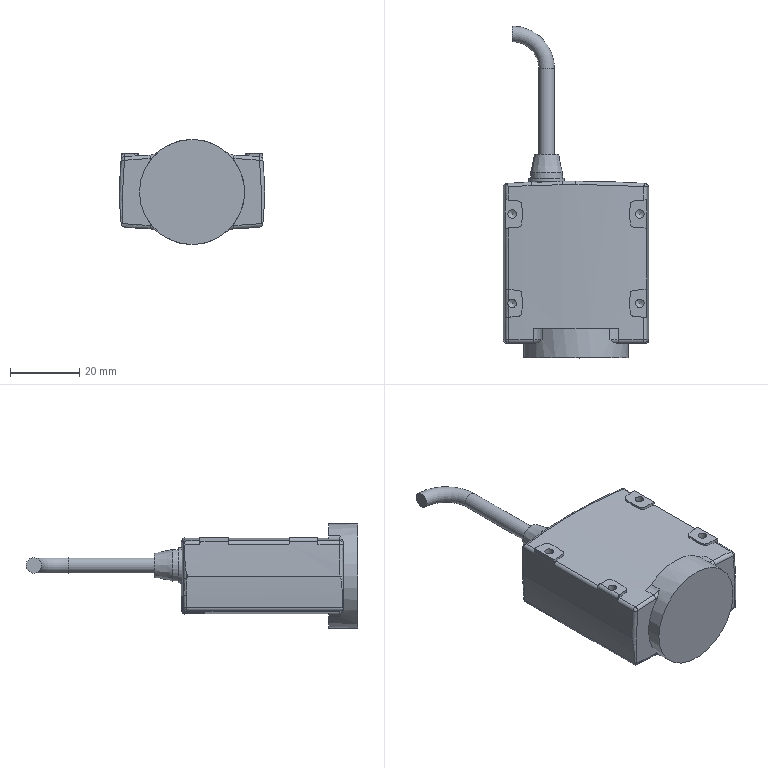Part | NX | features 5003_101_Code reader 2 | 1 solid | 283 faces | box 42.142 x 96.07 x 30.4 mm | volume 45672 mm3 | cylinder 105 | spline 86 | plane 60 | torus 21 | sphere 6 | cone 5 | commonest cylinder face diameters 0.4 x64 2 x9 2.013 x8 2.5 x4 8 x4 40.013 x4